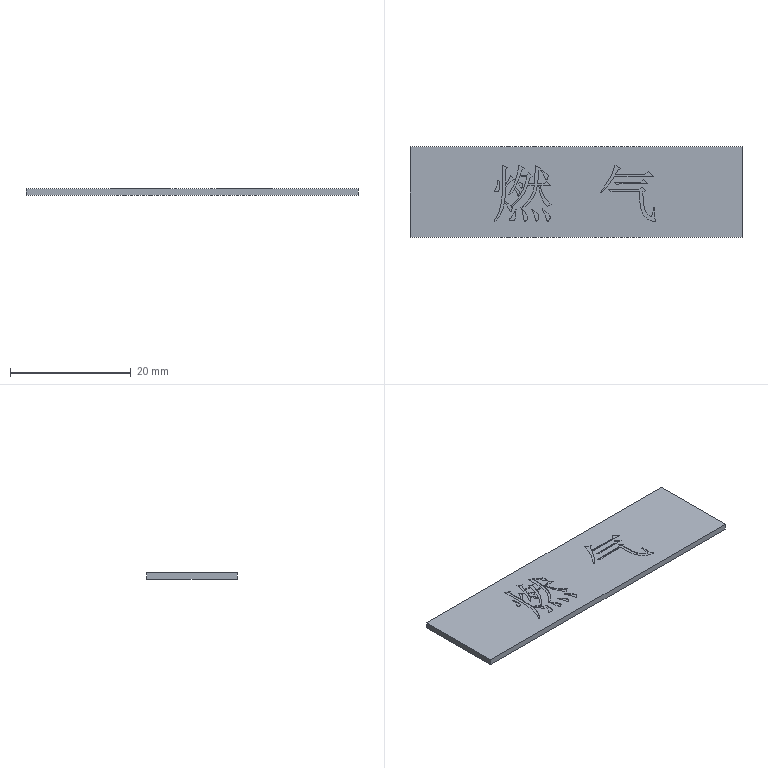Part | STEP file | HXGR200008-06-02-04 | 1 solid | 132 faces | box 55 x 15 x 1 mm | volume 821.434 mm3 | plane 67 | spline 65